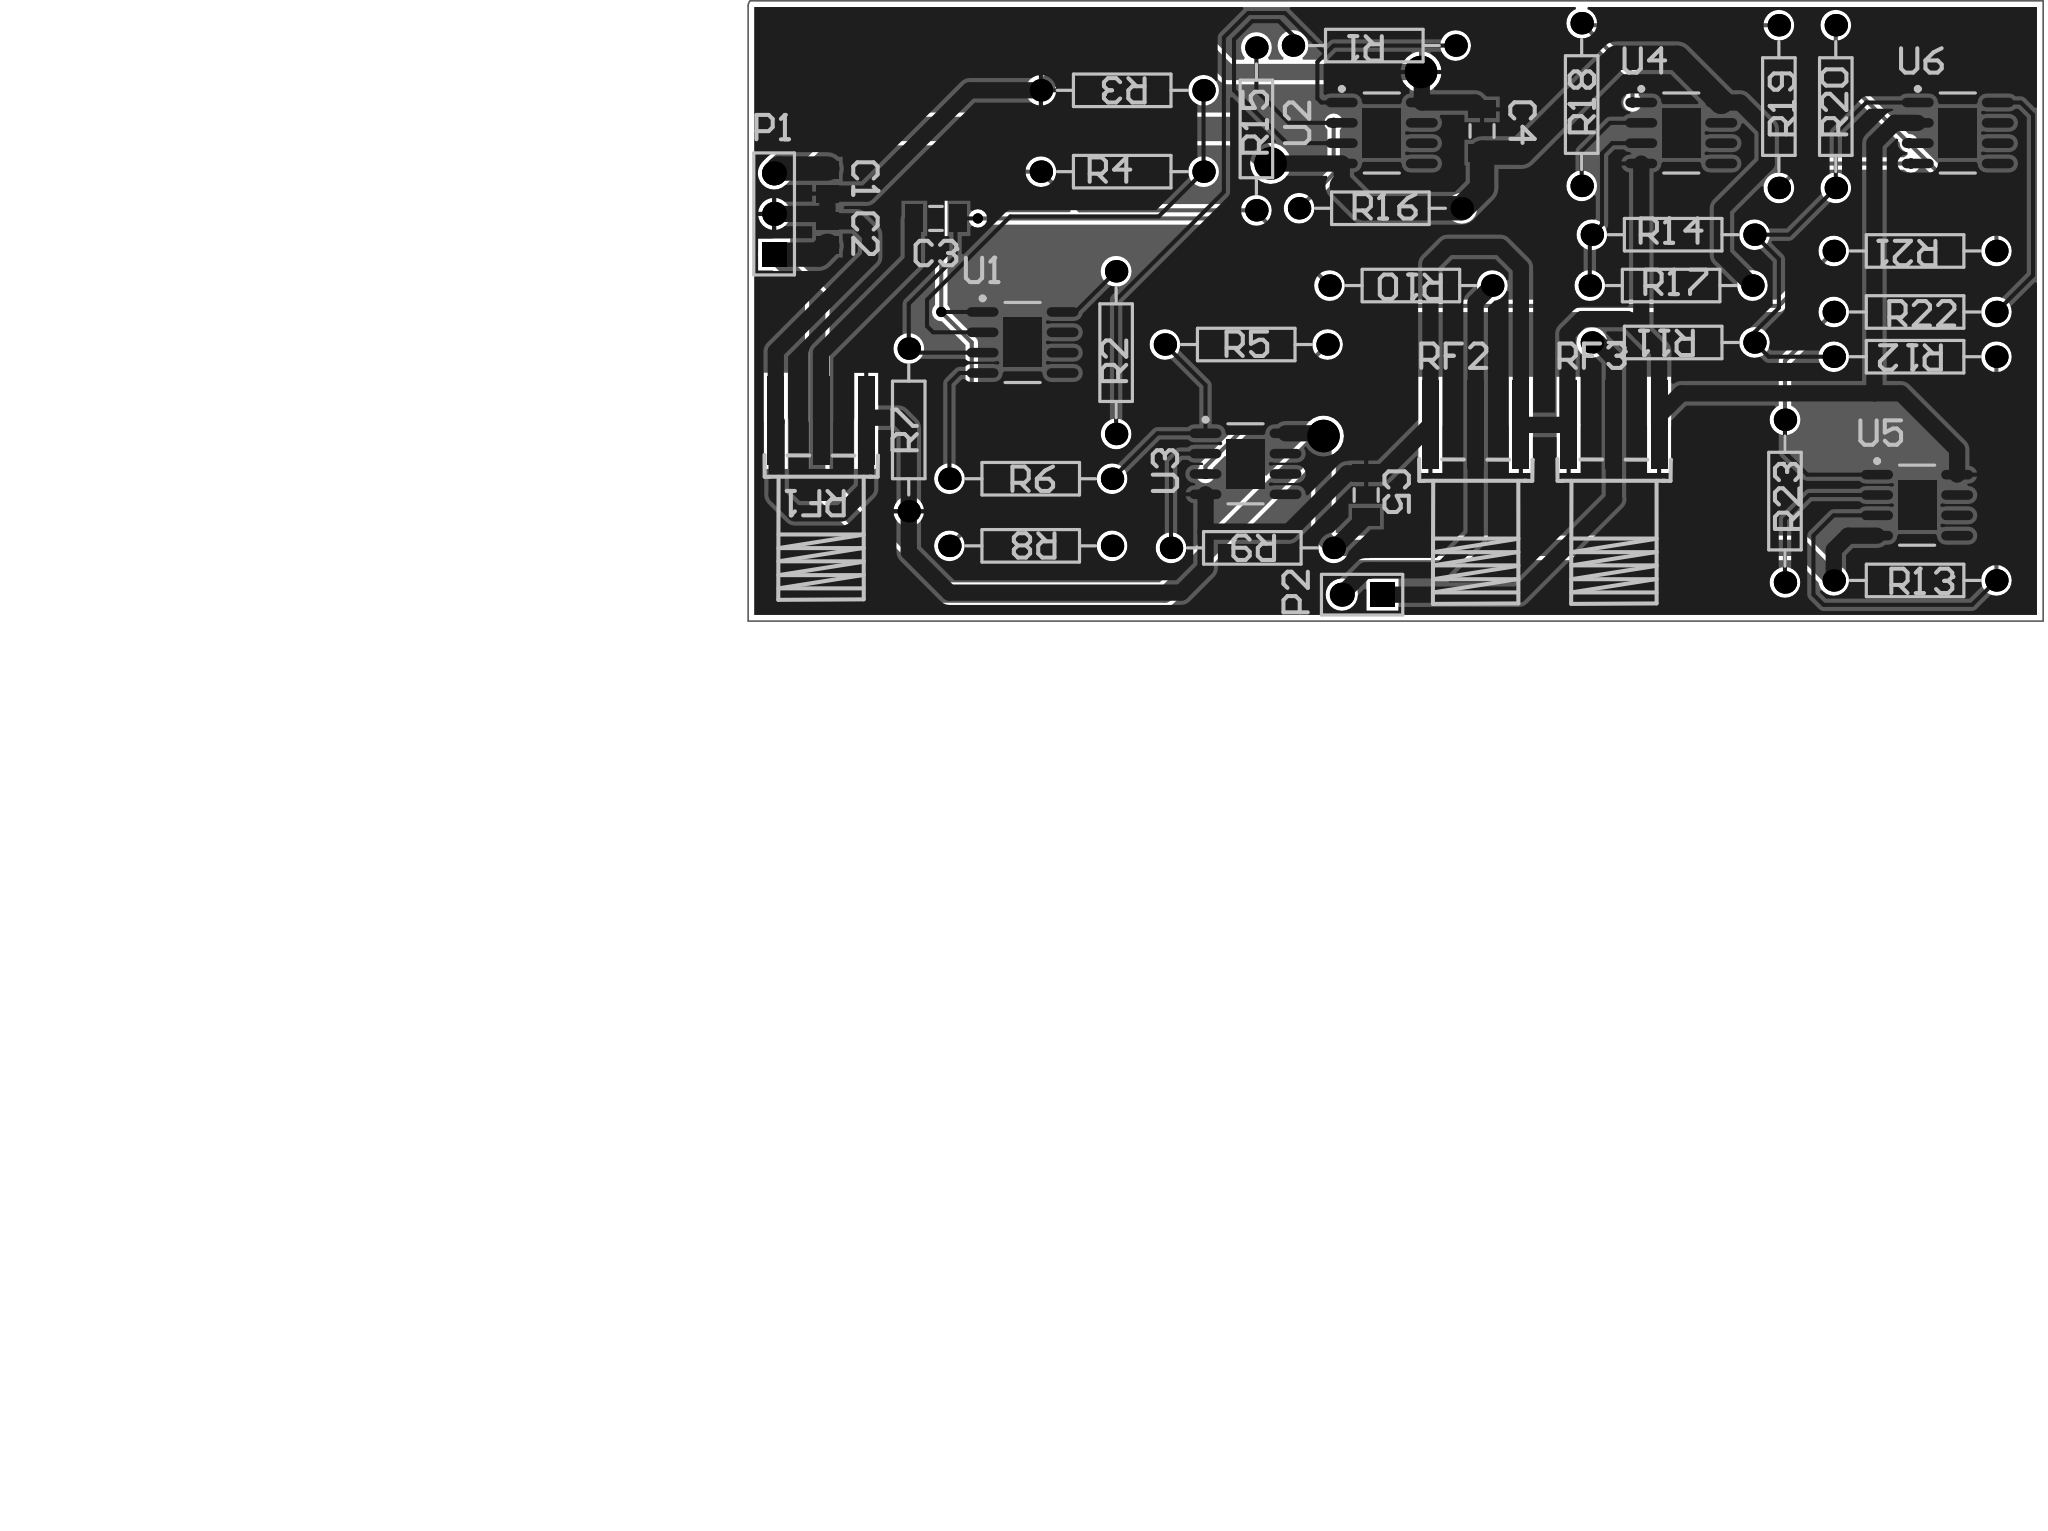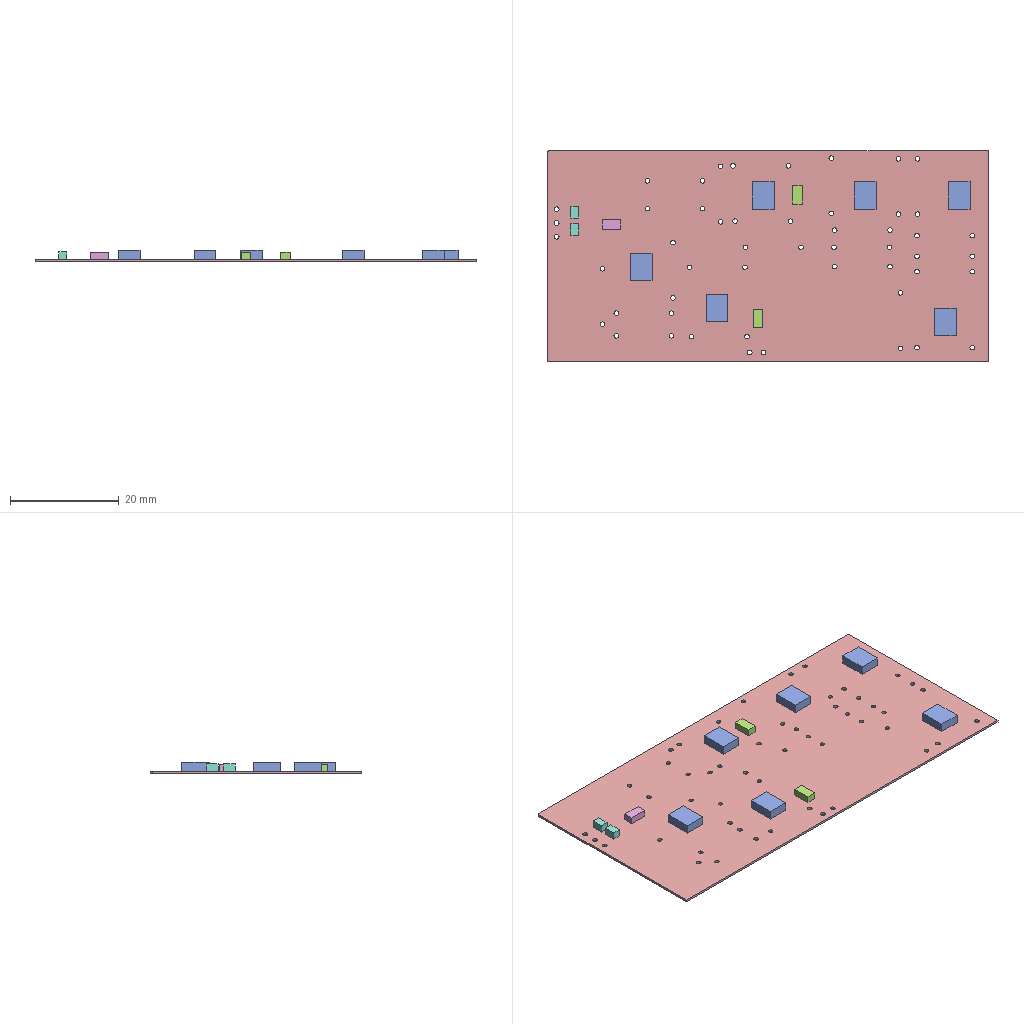Circuit board layout | Altium Designer | box 80.9 x 38.7 x 2.1 mm
Layer stack:
# Altium Designer layer stack of 3 (unit mm; dielectric type: 0 none, 1 core, 2 prepreg, 3 surface material)
index,name,kind,layer,copper_thickness_mm,dielectric_type,dielectric_thickness_mm,dielectric_material,dielectric_constant
0,Top Paste,other,,,,,,
1,Top Overlay,other,,,,,,
2,Top Solder,dielectric,,,3,0.0102,Solder Resist,3.5
3,Top Layer,copper,Top Layer,0.0356,,,,
4,Dielectric 1,dielectric,,,0,0.32,FR-4,4.8
5,Bottom Layer,copper,Bottom Layer,0.0356,,,,
6,Bottom Solder,dielectric,,,3,0.0102,Solder Resist,3.5
7,Bottom Overlay,other,,,,,,
8,Bottom Paste,other,,,,,,
# drill layer pairs: low layer,high layer
drill_pair,Top Layer,Bottom Layer
Part placement:
Designator,Comment,Layer,Footprint,Center-X(mm),Center-Y(mm),Rotation
U6,LM7372MR,TopLayer,MRA08B_N,122.301,86.995,0
U5,LM7372MR,TopLayer,MRA08B_N,119.761,63.754,0
U4,LM7372MR,TopLayer,MRA08B_N,105.029,86.995,0
U3,LM7372MR,TopLayer,MRA08B_N,77.806,66.337,0
U2,LM7372MR,TopLayer,MRA08B_N,86.32,86.995,0
U1,LM7372MR,TopLayer,MRA08B_N,63.881,73.914,0
RF3,SMA,TopLayer,SMA-SMD_HJ-SMA313,100.818,68.768,0
RF2,SMA,TopLayer,SMA-SMD_HJ-SMA313,92.182,68.768,0
RF1,SMA,TopLayer,SMA-SMD_HJ-SMA313,51.288,69.022,360
R23,10K,TopLayer,AXIAL-0.4,111.506,64.008,90
R22,1,TopLayer,AXIAL-0.4,119.634,75.819,360
R21,10K,TopLayer,AXIAL-0.4,119.634,79.629,180
R20,51K,TopLayer,AXIAL-0.4,114.681,88.646,90
R19,1,TopLayer,AXIAL-0.4,111.125,88.646,90
R18,100K,TopLayer,AXIAL-0.4,98.806,88.773,90
R17,100K,TopLayer,AXIAL-0.4,104.394,77.47,360
R16,100K,TopLayer,AXIAL-0.4,86.233,82.296,360
R15,100K,TopLayer,AXIAL-0.4,78.486,87.249,90
R14,100K,TopLayer,AXIAL-0.4,104.521,80.645,180
R13,100K,TopLayer,AXIAL-0.4,119.634,59.055,360
R12,100K,TopLayer,AXIAL-0.4,119.634,73.025,180
R11,50,TopLayer,AXIAL-0.4,104.521,73.914,180
R10,50,TopLayer,AXIAL-0.4,88.138,77.47,180
R9,100K,TopLayer,AXIAL-0.4,78.232,61.087,180
R8,100K,TopLayer,AXIAL-0.4,64.389,61.214,180
R7,1K,TopLayer,AXIAL-0.4,56.769,68.453,90
R6,1,TopLayer,AXIAL-0.4,64.389,65.405,180
R5,10K,TopLayer,AXIAL-0.4,77.851,73.787,360
R4,51k,TopLayer,AXIAL-0.4,70.104,84.582,180
R3,10K,TopLayer,AXIAL-0.4,70.104,89.662,360
R2,1,TopLayer,AXIAL-0.4,69.723,73.279,270
R1,10K,TopLayer,AXIAL-0.4,85.852,92.456,180
P2,Header 2,TopLayer,HDR1X2,85.09,58.166,180
P1,Header 3,TopLayer,HDR1X3,48.36,81.942,90
C5,104,TopLayer,C1206,85.344,64.389,270
C4,104,TopLayer,C1206,92.583,87.122,270
C3,104,TopLayer,C1206,58.467,81.661,180
C2,100UF/100V,TopLayer,C0805,51.689,80.772,270
C1,100UF/100V,TopLayer,C0805,51.689,83.959,270
Pad and via stacks:
# Altium Designer via and pad stacks of 3 (unit mm). Each distinct definition once, with the count of objects using it.
# via: kind,start_layer,end_layer,hole_mm,diameter_mm,mode(0 simple;1 top-mid-bottom;2 full stack),diameter_per_layer,count,example_net
# pad: kind,layer,hole_mm,hole_type(0 round;1 square;2 slot),plating,top_size,top_shape(1 round;2 rect;3 octagon;9 rounded rect),mid_size,bottom_size,mode,footprint,size_per_layer,count,example
pad,Top Layer,0,0,plated,1.7x1.1,2,1.7x1.1,1.7x1.1,0,C1206,,6,C5.1
pad,Top Layer,0,0,plated,1x5.5,2,1x5.5,1x5.5,0,SMA-SMD_HJ-SMA313,,9,RF2.3
pad,Top Layer,0,0,plated,2.41x3.1,2,2.41x3.1,2.41x3.1,0,MRA08B_N,,6,U3.9
pad,Top Layer,0,0,plated,0.6x2,1,0.6x2,0.6x2,0,MRA08B_N,,48,U3.5
pad,Top Layer,0,0,plated,1.4x1.1,2,1.4x1.1,1.4x1.1,0,C0805,,4,C2.1
pad,Multi-Layer,0.9,0,plated,1.5x1.5,1,1.5x1.5,1.5x1.5,0,HDR1X2,,1,P2.2
pad,Multi-Layer,0.9,0,plated,1.5x1.5,2,1.5x1.5,1.5x1.5,0,HDR1X2,,1,P2.1
pad,Multi-Layer,0.85,0,plated,1.4x1.4,1,1.4x1.4,1.4x1.4,0,AXIAL-0.4,,46,R9.2
pad,Multi-Layer,0.9,0,plated,1.5x1.5,1,1.5x1.5,1.5x1.5,0,HDR1X3,,2,P1.3
pad,Multi-Layer,0.9,0,plated,1.5x1.5,2,1.5x1.5,1.5x1.5,0,HDR1X3,,1,P1.1
pad,Bottom Layer,0,0,plated,1x5.5,2,1x5.5,1x5.5,0,SMA-SMD_HJ-SMA313,,6,RF2.4
via,Top Layer,Bottom Layer,0.33,0.66,0,,24,
via,Top Layer,Bottom Layer,0.381,0.635,0,,7,NetR4_2
via,Top Layer,Bottom Layer,1.143,2.032,0,,3,VCC
Copper pours:
name,layer,net,type(0 solid;1 hatched;2 none)
Top Layer-No Net,Bottom Layer,GND,0
Top Layer-No Net,Top Layer,GND,0
Design rules, without the lines most boards share:
# Altium Designer design rules of 3 (exported by Altium Designer, unit mm)
# columns: name | kind | enabled | priority | scope1 | scope2 | descriptor | typed fields (field=value)
HoleToHoleClearance | 52 | enabled | 1 | All | All | Hole To Hole Clearance (Gap=10mil) (All),(All) | gap=0.254
DiffPairsRouting | 51 | enabled | 1 | All | All | Differential Pairs Uncoupled Length using the Gap Constraints (Min=10mil) (Max=10mil) (Prefered=10mil)  and Width Constraints (Min=15mil) (Max=15mil) (Prefered=15mil) (All) |
SolderMaskExpansion | 13 | enabled | 1 | All | All | Solder Mask Expansion (Expansion =4mil) (All) | expansion=0.1016
PasteMaskExpansion | 14 | enabled | 1 | All | All | Paste Mask Expansion (Expansion =0mil) (All) | expansion=0
RoutingVias | 11 | enabled | 1 | All | All | Routing Via (MinHoleWidth=28mil) (MaxHoleWidth=28mil) (PreferredHoleWidth=28mil) (MinWidth=50mil) (MaxWidth=50mil) (PreferedWidth=50mil) (All) | via_min_hole=0.7112 via_max_hole=0.7112 via_preferred_diameter=1.27 via_preferred_hole=0.7112
Width | 2 | enabled | 1 | All | All | Width Constraint (Min=10mil) (Max=1000mil) (Preferred=10mil) (All) |
PolygonConnect | 20 | enabled | 1 | All | All | Polygon Connect Rule(Relief Connect )(Conductor Width=10mil) (Relief Angle=90 Angle) (Entries=4) (Air Gap Width=10mil) (All),(All) | connect_style(0=relief,1=direct,2=none)=0 relief_conductor_width=0.254 relief_entries=4
PlaneConnect | 6 | enabled | 1 | All | All | Power Plane Connect Rule(Relief Connect )(Expansion=20mil) (Conductor Width=10mil) (Air Gap=10mil) (Entries=4) (All) | relief_conductor_width=0.254 relief_entries=4 relief_expansion=0.508
Clearance | 0 | enabled | 1 | All | All | Clearance Constraint (Gap=10mil) (All),(All) | gap=0.254
Classes set for this board:
# Altium Designer classes of 3 (member kind: 0 net, 1 component, 2 from-to, 3 pad, 4 layer, 5 differential pair, 6 design channel, 7 polygon, 8 structure, 9 xSignal)
# columns: class name | member kind | superclass | members
Sheet1 | 1 | no | C1; C2; C3; C4; C5; P1; P2; R1; R2; R3; R4; R5; R6; R7; R8; R9; R10; R11; R12; R13; R14; R15; R16; R17; R18; R19; R20; R21; R22; R23; RF1; RF2; RF3; U1; U2; U3; U4; U5; U6;